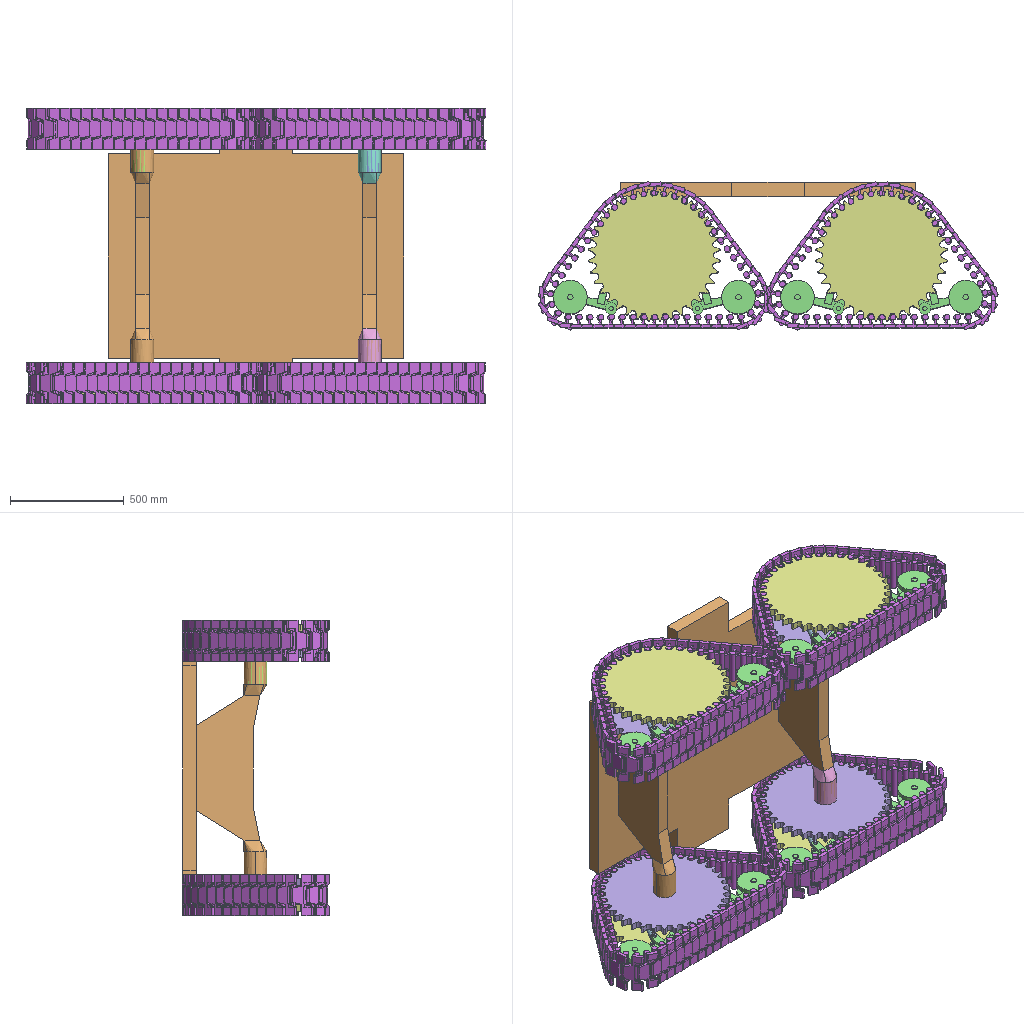Assembly | SolidWorks | 11 different items | 240 placed | box 2024 x 649 x 1300 mm
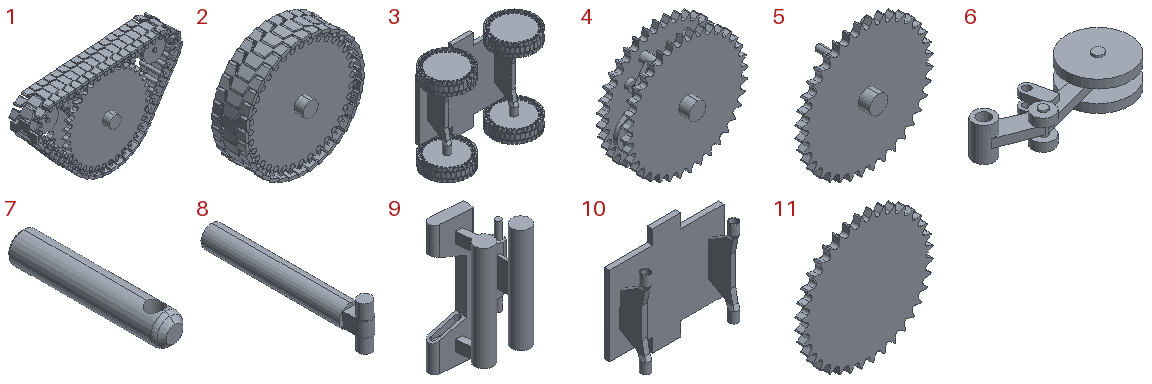Parts list (item | name | quantity | parent item | size | volume | features):
1 | (subassembly) | x4 | - | - | 31623376 mm3 | features ReferencePattern 84, CompositeCurve 2, LocalChainPattern 1, LocalCirPattern 1, RefAxis 1
2 | (subassembly) | x1 | - | 643.603 x 212.5 x 643.603 mm | 27651397 mm3 | features ReferencePattern 70, CompositeCurve 4, LocalCirPattern 2, RefAxis 1
3 | (subassembly) | x1 | - | - | 206829671 mm3 | -
4 | (subassembly) | x1 | - | 579.141 x 195 x 579.141 mm | 17437736 mm3 | features CompositeCurve 2, RefAxis 1
5 | - | x4 | in 1 | 577.823 x 165 x 577.823 mm | 7420375 mm3 | features ICE 3, Extrusion 1
6 | - | x8 | in 1 | 370 x 150 x 80 mm | 1159902 mm3 | features ICE 4, Extrusion 1, MirrorSolid 1
7 | - | x8 | in 1 | 45 x 230 x 45 mm | 210439 mm3 | features ICE 3, Chamfer 2, Extrusion 1, Fillet 1
8 | - | x8 | in 1 | 30 x 220 x 60 mm | 155623 mm3 | features ICE 2, Extrusion 1
9 | - | x200 | in 1 | 97.078 x 65.941 x 180 mm | 283713 mm3 | features ICE 6, RefPoint 4, Fillet 2, Extrusion 1, MirrorPattern 1
10 | - | x1 | - | 1300 x 370 x 1220 mm | 96223976 mm3 | features ICE 3, MirrorSolid 2, Blend 1, Extrusion 1, LPattern 1, MirrorPattern 1, RefPoint 1
11 | - | x4 | in 1 | 577.823 x 30 x 577.823 mm | 6965433 mm3 | features ICE 2, Extrusion 1
Mates (type | each side: item.copy, entity, surface, feature):
In the top assembly
Concentric | 10.1 face cylinder LPattern1 | 5.1 face cylinder Boss-Extrude3
Coincident | 10.1 face plane LPattern1 | 5.1 face plane Boss-Extrude1
Parallel | 10.1 face plane Boss-Extrude2 | 9.1 face plane Boss-Extrude2
Concentric | 10.1 face cylinder LPattern1 | 5.2 face cylinder Boss-Extrude3
Coincident | 10.1 face plane LPattern1 | 5.2 face plane Boss-Extrude1
Parallel | 10.1 face plane Boss-Extrude2 | 9.2 face plane Boss-Extrude2
Concentric | 10.1 face cylinder Boss-Extrude1 | 5.3 face cylinder Boss-Extrude3
Coincident | 10.1 face plane Boss-Extrude1 | 5.3 face plane Boss-Extrude1
Parallel | 10.1 face plane Boss-Extrude2 | 9.3 face plane Boss-Extrude2
Concentric | 10.1 face cylinder Boss-Extrude1 | 5.4 face cylinder Boss-Extrude3
Coincident | 10.1 face plane Boss-Extrude1 | 5.4 face plane Boss-Extrude1
Parallel | 10.1 face plane Boss-Extrude2 | 9.4 face plane Boss-Extrude2
In subassembly 1
Concentric | 5.5 face cylinder Boss-Extrude2 | 6.1 face cylinder Boss-Extrude1
DistanceDim | 5.5 face plane Boss-Extrude1 | 6.1 face plane Boss-Extrude1
Concentric | 5.5 face cylinder Boss-Extrude2 | 6.2 face cylinder Boss-Extrude1
DistanceDim | 5.5 face plane Boss-Extrude2 | 6.2 face plane Boss-Extrude1
Concentric | 5.5 face cylinder Boss-Extrude2 | 7.1 face cylinder Cut-Extrude2
Concentric | 5.5 face cylinder Boss-Extrude2 | 7.2 face cylinder Cut-Extrude2
DistanceDim | 5.5 face plane Boss-Extrude1 | 7.1 plane
DistanceDim | 5.5 face plane Boss-Extrude1 | 7.2 plane
Concentric | 6.1 face cylinder Boss-Extrude5 | 8.1 face cylinder Boss-Extrude3
Concentric | 7.2 face cylinder Cut-Extrude1 | 8.1 face cylinder Boss-Extrude1
Concentric | 7.1 face cylinder Cut-Extrude1 | 8.2 face cylinder Boss-Extrude1
Concentric | 6.2 face cylinder Mirror2 | 8.2 face cylinder Boss-Extrude3
Coincident | 5.5 face plane Cut-Extrude1 | 11.1 face plane Cut-Extrude1
Concentric | 5.5 select_type:24 | 11.1 select_type:24
Coincident | 5.5 face plane Boss-Extrude2 | 11.1 face plane Boss-Extrude1
Coincident | 5.5 select_type:25 | 1.1 axis
Parallel | 6.2 select_type:24 | 1.1 select_type:10
Parallel | 6.1 select_type:24 | 1.1 select_type:10